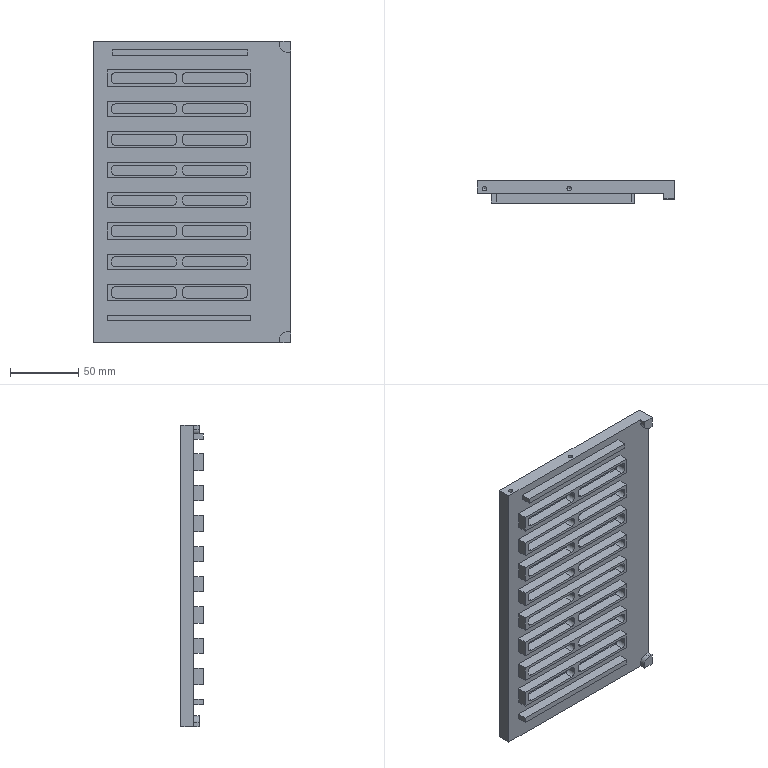NC program | NX | posted with a generic post | part box 144.5 x 16.5 x 221 mm
Lines 25 to 834 of 8751:
(动态加工0.5 , TOOL : D8-25-D8-60-3T-ROUGH)
N48 T02 M6
N50 G53
N52 G17 G0 G90 X-126.572 Y2.423 B0. C0. S6000 M3
N54 G43 Z20. H2
N56 Z-12.
N58 G94 G1 X-126.422 Y2.436 Z-12.937 F3500.
N60 X-126.273 Y2.448 Z-13.308
N62 X-126.123 Y2.46 Z-13.58
N64 X-125.974 Y2.473 Z-13.8
N66 X-125.824 Y2.485 Z-13.984
N68 X-125.675 Y2.497 Z-14.142
N70 X-125.525 Y2.509 Z-14.28
N72 X-125.376 Y2.522 Z-14.4
N74 X-125.226 Y2.534 Z-14.505
N76 X-125.077 Y2.546 Z-14.598
N78 X-124.927 Y2.559 Z-14.679
N80 X-124.778 Y2.571 Z-14.75
N82 X-124.628 Y2.583 Z-14.81
N84 X-124.479 Y2.596 Z-14.862
N86 X-124.329 Y2.608 Z-14.905
N88 X-124.18 Y2.62 Z-14.939
N90 X-124.03 Y2.632 Z-14.966
N92 X-123.881 Y2.645 Z-14.985
N94 X-123.731 Y2.657 Z-14.996
N96 X-123.582 Y2.669 Z-15.
N98 X-122.198 Y2.783
N100 G3 X-121.548 Y3.214 R0.809
N102 X-120.82 Y5.812 R7.175
N104 X-120.527 Y11.884 R57.317
N106 G1 X-120.499 Y20.852
N108 X-120.498 Y76.502
N110 G2 X-119.038 Y79.444 R4.189
N112 X-115.307 Y81.289 R8.348
N114 X-109.801 Y81.906 R27.841
N116 X-97.202 Y81.998 R442.635
N118 G1 X115.027 Y81.997
N120 G2 X118.015 Y80.473 R4.207
N122 X119.814 Y76.725 R8.506
N124 X120.407 Y71.291 R28.543
N126 X120.498 Y58.767 R445.831
N128 G1 Y-76.524
N130 G2 X118.974 Y-79.512 R4.21
N132 X115.292 Y-81.296 R8.462
N134 X109.785 Y-81.907 R28.074
N136 X97.261 Y-81.998 R443.425
N138 G1 X-115.074 Y-81.996
N140 G2 X-118.046 Y-80.436 R4.252
N142 X-119.809 Y-76.741 R8.541
N144 X-120.406 Y-71.308 R28.316
N146 X-120.498 Y-58.783 R440.931
N148 G1 X-120.497 Y0.042
N150 G2 X-120.074 Y3.928 R35.862
N152 G3 X-119.543 Y12.571 R72.923
N154 X-119.499 Y22.428 R692.354
N156 G1 X-119.498 Y73.828
N158 G2 X-117.119 Y78.386 R5.853
N160 X-112.81 Y80.274 R10.684
N162 X-106.701 Y80.904 R34.296
N164 X-94.327 Y80.997 R453.189
N166 G1 X112.476 Y80.994
N168 G2 X116.942 Y78.556 R5.865
N170 X118.82 Y74.1 R10.921
N172 X119.416 Y67.837 R36.785
N174 X119.498 Y55.387 R532.275
N176 G1 X119.494 Y-73.973
N178 G2 X117.007 Y-78.477 R5.893
N180 X112.541 Y-80.332 R11.039
N182 X106.276 Y-80.918 R37.482
N184 X93.827 Y-80.997 R545.572
N186 G1 X-112.473 Y-80.994
N188 G2 X-116.98 Y-78.505 R5.892
N190 X-118.833 Y-74.038 R11.051
N192 X-119.42 Y-67.698 R37.896
N194 X-119.498 Y-55.248 R562.114
N196 G1 X-119.497 Y-2.098
N198 G2 X-119.043 Y3.975 R62.156
N200 G3 X-118.518 Y16.146 R127.55
N202 G1 X-118.499 Y24.377
N204 X-118.497 Y71.577
N206 G2 X-115.243 Y77.527 R6.962
N208 X-110.43 Y79.342 R12.909
N210 X-103.862 Y79.917 R42.826
N212 X-91.113 Y79.997 R580.954
N214 G1 X110.062 Y79.996
N216 G2 X115.98 Y76.819 R6.934
N218 X117.811 Y72.095 R12.632
N220 X118.419 Y65.304 R42.014
N222 X118.497 Y52.555 R594.339
N224 G1 Y-71.52
N226 G2 X115.257 Y-77.521 R6.958
N228 X110.437 Y-79.34 R12.859
N230 X103.869 Y-79.916 R42.675
N232 X91.044 Y-79.997 R572.005
N234 G1 X-109.981
N236 G2 X-116.086 Y-76.658 R6.99
N238 X-117.847 Y-71.902 R13.06
N240 X-118.417 Y-65.333 R42.909
N242 X-118.497 Y-52.959 R565.196
N244 G1 X-118.496 Y-3.823
N246 G2 X-118.029 Y4.001 R89.068
N248 G3 X-117.515 Y17.567 R166.648
N250 G1 X-117.5 Y25.802
N252 X-117.498 Y69.402
N254 G2 X-116.518 Y73.666 R8.362
N256 X-112.306 Y77.273 R8.771
N258 X-106.93 Y78.592 R18.736
N260 X-98.543 Y78.972 R83.321
N262 G1 X-88.643 Y78.997
N264 X107.901 Y78.996
N266 G2 X112.032 Y78.093 R8.448
N268 X115.653 Y74.066 R8.574
N270 X117.076 Y68.568 R18.105
N272 X117.471 Y60.181 R80.674
N274 G1 X117.497 Y50.281
N276 X117.496 Y-69.398
N278 G2 X116.595 Y-73.53 R8.459
N280 X112.602 Y-77.139 R8.605
N282 X107.184 Y-78.561 R17.911
N284 X99.398 Y-78.962 R73.9
N286 G1 X88.673 Y-78.997
N288 X-107.974 Y-78.996
N290 G2 X-112.355 Y-77.908 R8.215
N292 X-115.794 Y-73.751 R8.867
N294 X-117.123 Y-68.148 R19.381
N296 X-117.471 Y-60.133 R86.468
N298 G1 X-117.497 Y-50.233
N300 X-117.496 Y-5.283
N302 G2 X-117.03 Y3.898 R114.608
N304 G3 X-116.507 Y20.185 R214.532
N306 G1 X-116.5 Y26.777
N308 X-116.497 Y67.677
N310 G2 X-115.77 Y71.707 R9.891
N312 X-114.392 Y73.841 R8.626
N314 X-113.812 Y74.84 R9.182
N316 G1 X-113.166 Y75.506
N318 X-112.382 Y76.016
N320 G2 X-104.826 Y77.671 R26.45
N322 X-94.784 Y77.982 R129.687
N324 G1 X-86.234 Y77.996
N326 X105.941 Y77.995
N328 G2 X109.85 Y77.416 R10.756
N330 X112.046 Y76.145 R8.329
N332 X114.414 Y73.807 R4.347
N334 X116.017 Y67.661 R21.369
N336 X116.455 Y59.576 R76.219
N338 X116.497 Y47.952 R776.314
N340 G1 X116.496 Y-67.423
N342 G2 X115.925 Y-71.334 R10.852
N344 X114.389 Y-73.845 R8.349
N346 X113.795 Y-74.854 R8.385
N348 G1 X113.129 Y-75.525
N350 X112.331 Y-76.03
N352 G2 X104.54 Y-77.691 R27.089
N354 X95.097 Y-77.981 R129.679
N356 G1 X85.647 Y-77.996
N358 X-105.928 Y-77.995
N360 G2 X-109.838 Y-77.421 R10.811
N362 X-112.065 Y-76.134 R8.669
N364 X-113.117 Y-75.535 R5.064
N366 G1 X-113.431 Y-75.318
N368 G2 X-114.645 Y-73.254 R6.134
N370 X-116.102 Y-66.911 R23.207
N372 X-116.475 Y-57.847 R98.48
N374 G1 X-116.497 Y-48.772
N376 X-116.495 Y-6.448
N378 G2 X-115.991 Y4.399 R154.223
N380 G3 X-115.507 Y22.284 R267.315
N382 G1 X-115.5 Y29.478
N384 X-115.499 Y65.428
N386 G2 X-115.121 Y69.297 R14.61
N388 G1 X-114.705 Y70.58
N390 G2 X-114.674 Y72.714 R53.083
N392 X-114.306 Y74.023 R5.537
N394 G1 X-114.597 Y73.172
N396 G3 X-114.7 Y72.25 R4.874
N398 G2 X-114.826 Y67.431 R63.555
N400 G3 X-114.9 Y56.482 R427.272
N402 G1 X-114.902 Y26.224
N404 G2 X-115.149 Y8.97 R408.984
N406 X-115.735 Y-1.084 R927.803
N408 G3 X-115.895 Y-10.982 R203.441
N410 G1 X-115.896 Y-69.082
N412 X-115.907 Y-69.211
N414 X-115.938 Y-69.338
N416 X-115.99 Y-69.457
N418 X-116.87 Y-70.751 Z-14.8
N420 X-117.517 Y-71.697 F15000.
N422 G3 X-117.656 Y-72.13 R0.814
N424 G1 X-117.68 Y-73.17
N426 G3 X-117.306 Y-73.866 R0.801
N428 G1 X-116.187 Y-74.568
N430 X-115.775 Y-74.83 Z-14.862 F3500.
N432 X-115.356 Y-75.079 Z-14.925
N434 G3 X-114.781 Y-75.106 Z-15. R0.82
N436 X-114.28 Y-74.081 R0.8
N438 G1 X-114.594 Y-73.189
N440 G2 X-114.709 Y-71.121 R12.101
N442 X-114.891 Y-62.061 R153.374
N444 G1 X-114.896 Y-55.461
N446 Y66.539
N448 G3 X-115.166 Y67.138 R0.803
N450 X-115.993 Y67.285 Z-14.887 R0.828
N452 G1 X-116.648 Y67.094 Z-14.8
N454 X-117.85 Y66.742 F15000.
N456 G2 X-117.945 Y68.299 R-0.8
N458 G3 X-117.48 Y68.268 R1.327
N460 X-116.877 Y68.756 R0.801
N462 G1 X-116.667 Y69.276
N464 X-116.437 Y69.853 Z-14.879 F3500.
N466 X-116.195 Y70.424 Z-14.959
N468 X-116.099 Y70.554 Z-14.979
N470 X-115.983 Y70.665 Z-15.
N472 G2 X-114.7 Y70.027 R0.8
N474 G1 Y-72.25
N476 X-114.594 Y-73.189
N478 G3 X-113.907 Y-74.735 R5.716
N480 G1 X-113.431 Y-75.318
N482 X-112.321 Y-76.035
N484 G3 X-105.433 Y-77.31 R20.765
N486 X-94.184 Y-77.396 R367.013
N488 G1 X107.316
N490 X107.446 Y-77.407
N492 X107.572 Y-77.438
N494 X107.692 Y-77.49
N496 G2 X108.119 Y-78.223 Z-14.886 R0.827
N498 G1 X108.159 Y-78.894 Z-14.8
N500 X108.232 Y-80.132 F15000.
N502 G3 X109.805 Y-79.885 R-0.8
N504 G1 X109.724 Y-79.575
N506 X109.657 Y-79.262
N508 G2 X110.257 Y-78.415 R0.813
N510 G1 X111.739 Y-77.912 Z-15. F3500.
N512 G3 X111.439 Y-76.344 R0.801
N514 G1 X110.499 Y-76.45
N516 X-110.501
N518 X-111.578 Y-76.344
N520 X-114.012 Y-76.94
N522 G2 X-114.793 Y-76.715 R0.809
N524 G1 X-114.897 Y-76.606 Z-14.996
N526 X-115.001 Y-76.498 Z-14.985
N528 X-115.104 Y-76.39 Z-14.966
N530 X-115.208 Y-76.281 Z-14.939
N532 X-115.312 Y-76.173 Z-14.905
N534 X-115.415 Y-76.064 Z-14.862
N536 X-115.519 Y-75.956 Z-14.81
N538 X-115.623 Y-75.847 Z-14.75
N540 X-115.726 Y-75.739 Z-14.679
N542 X-115.83 Y-75.63 Z-14.598
N544 X-115.933 Y-75.522 Z-14.505
N546 X-116.037 Y-75.414 Z-14.4
N548 X-116.141 Y-75.305 Z-14.28
N550 X-116.244 Y-75.197 Z-14.142
N552 X-116.348 Y-75.088 Z-13.984
N554 X-116.452 Y-74.98 Z-13.8
N556 X-116.555 Y-74.871 Z-13.58
N558 X-116.659 Y-74.763 Z-13.308
N560 X-116.763 Y-74.655 Z-12.937
N562 X-116.866 Y-74.546 Z-12.
N564 G0 Z20.
N566 X-110.132 Y78.917
N568 Z-12.
N570 G1 X-110.273 Y78.866 Z-12.937
N572 X-110.414 Y78.814 Z-13.308
N574 X-110.555 Y78.763 Z-13.58
N576 X-110.696 Y78.712 Z-13.8
N578 X-110.837 Y78.66 Z-13.984
N580 X-110.978 Y78.609 Z-14.142
N582 X-111.119 Y78.558 Z-14.28
N584 X-111.26 Y78.506 Z-14.4
N586 X-111.401 Y78.455 Z-14.505
N588 X-111.542 Y78.404 Z-14.598
N590 X-111.683 Y78.352 Z-14.679
N592 X-111.824 Y78.301 Z-14.75
N594 X-111.965 Y78.25 Z-14.81
N596 X-112.106 Y78.198 Z-14.862
N598 X-112.247 Y78.147 Z-14.905
N600 X-112.388 Y78.096 Z-14.939
N602 X-112.528 Y78.044 Z-14.966
N604 X-112.669 Y77.993 Z-14.985
N606 X-112.81 Y77.942 Z-14.996
N608 X-112.951 Y77.89 Z-15.
N610 G3 X-112.67 Y76.323 R0.808
N612 X-110.538 Y76.45 R10.828
N614 X-105.599 Y76.621 R42.041
N616 G2 X-92.557 Y76.984 R193.286
N618 G1 X-83.707 Y76.996
N620 X106.093 Y76.988
N622 G2 X108.504 Y76.455 R13.506
N624 G1 X110.501 Y76.45
N626 G2 X112.067 Y76.135 R4.094
N628 G3 X110.501 Y76.45 R4.094
N630 G1 X-108.2
N632 G2 X-108.545 Y76.527 R0.864
N634 G1 X-109.265 Y76.866
N636 G2 X-108.921 Y78.405 R0.808
N638 G1 X-108.771 Z-14.996
N640 X-108.621 Z-14.985
N642 X-108.471 Z-14.966
N644 X-108.321 Z-14.939
N646 X-108.171 Z-14.905
N648 X-108.021 Z-14.862
N650 X-107.871 Z-14.81
N652 X-107.721 Z-14.75
N654 X-107.571 Z-14.679
N656 X-107.421 Z-14.598
N658 X-107.271 Z-14.505
N660 X-107.121 Z-14.4
N662 X-106.971 Z-14.28
N664 X-106.821 Z-14.142
N666 X-106.671 Z-13.984
N668 X-106.521 Z-13.8
N670 X-106.371 Z-13.58
N672 X-106.221 Z-13.308
N674 X-106.071 Z-12.937
N676 X-105.921 Z-12.
N678 G0 Z20.
N680 X112.849 Y78.683
N682 Z-12.
N684 G1 X112.953 Y78.575 Z-12.937
N686 X113.056 Y78.466 Z-13.308
N688 X113.16 Y78.357 Z-13.58
N690 X113.263 Y78.249 Z-13.8
N692 X113.367 Y78.14 Z-13.984
N694 X113.47 Y78.032 Z-14.142
N696 X113.574 Y77.923 Z-14.28
N698 X113.677 Y77.814 Z-14.4
N700 X113.781 Y77.706 Z-14.505
N702 X113.884 Y77.597 Z-14.598
N704 X113.987 Y77.489 Z-14.679
N706 X114.091 Y77.38 Z-14.75
N708 X114.194 Y77.271 Z-14.81
N710 X114.298 Y77.163 Z-14.862
N712 X114.401 Y77.054 Z-14.905
N714 X114.505 Y76.946 Z-14.939
N716 X114.608 Y76.837 Z-14.966
N718 X114.712 Y76.728 Z-14.985
N720 X114.815 Y76.62 Z-14.996
N722 X114.919 Y76.511 Z-15.
N724 G2 X114.813 Y75.303 R0.808
N726 G1 X114.616 Y75.16
N728 X114.428 Y75.006
N730 G3 X114.255 Y74.146 R0.809
N732 G2 X114.7 Y72.589 R4.894
N734 G3 X114.91 Y68.872 R26.258
N736 G2 X115.47 Y56.739 R125.425
N738 G1 X115.496 Y45.49
N740 X115.489 Y-68.399
N742 G2 X114.718 Y-70.746 R15.407
N744 G3 X114.7 Y-72.756 R32.963
N746 G2 X114.323 Y-73.978 R4.614
N748 G3 X114.7 Y-72.756 R4.614
N750 G2 X114.814 Y-68.647 R44.469
N752 G3 X114.896 Y-57.548 R380.538
N754 G1 X114.888 Y67.402
N756 X114.7 Y68.1
N758 Y71.325
N760 Y-70.575
N762 G3 X115.489 Y-71.383 R0.808
N764 G1 X116.656 Y-71.41
N766 X116.806 Y-71.414 Z-14.996
N768 X116.956 Y-71.418 Z-14.985
N770 X117.106 Y-71.421 Z-14.966
N772 X117.256 Y-71.425 Z-14.939
N774 X117.406 Y-71.428 Z-14.905
N776 X117.556 Y-71.432 Z-14.862
N778 X117.706 Y-71.435 Z-14.81
N780 X117.855 Y-71.439 Z-14.75
N782 X118.005 Y-71.442 Z-14.679
N784 X118.155 Y-71.446 Z-14.598
N786 X118.305 Y-71.449 Z-14.505
N788 X118.455 Y-71.453 Z-14.4
N790 X118.605 Y-71.456 Z-14.28
N792 X118.755 Y-71.46 Z-14.142
N794 X118.905 Y-71.464 Z-13.984
N796 X119.055 Y-71.467 Z-13.8
N798 X119.205 Y-71.471 Z-13.58
N800 X119.355 Y-71.474 Z-13.308
N802 X119.505 Y-71.478 Z-12.937
N804 X119.655 Y-71.481 Z-12.
N806 G0 Z20.
N808 X3.098 Y-2.223
N810 Z3.
N812 G3 X3.098 Y-2.223 Z2.605 I-3.098 J1.833
N814 X3.098 Y-2.223 Z2.21 I-3.098 J1.833
N816 X3.098 Y-2.223 Z1.816 I-3.098 J1.833
N818 X3.098 Y-2.223 Z1.421 I-3.098 J1.833
N820 X3.098 Y-2.223 Z1.026 I-3.098 J1.833
N822 X3.098 Y-2.223 Z0.631 I-3.098 J1.833
N824 X3.098 Y-2.223 Z0.236 I-3.098 J1.833
N826 X3.098 Y-2.223 Z-0.159 I-3.098 J1.833
N828 X3.098 Y-2.223 Z-0.553 I-3.098 J1.833
N830 X3.098 Y-2.223 Z-0.948 I-3.098 J1.833
N832 X3.098 Y-2.223 Z-1.343 I-3.098 J1.833
N834 X3.098 Y-2.223 Z-1.738 I-3.098 J1.833
N836 X3.098 Y-2.223 Z-2.133 I-3.098 J1.833
N838 X3.098 Y-2.223 Z-2.528 I-3.098 J1.833
N840 X3.098 Y-2.223 Z-2.922 I-3.098 J1.833
N842 X3.098 Y-2.223 Z-3.317 I-3.098 J1.833
N844 X3.098 Y-2.223 Z-3.712 I-3.098 J1.833
N846 X3.098 Y-2.223 Z-4.107 I-3.098 J1.833
N848 X3.098 Y-2.223 Z-4.502 I-3.098 J1.833
N850 X3.098 Y-2.223 Z-4.896 I-3.098 J1.833
N852 X3.098 Y-2.223 Z-5.291 I-3.098 J1.833
N854 X3.098 Y-2.223 Z-5.686 I-3.098 J1.833
N856 X3.098 Y-2.223 Z-6.081 I-3.098 J1.833
N858 X3.098 Y-2.223 Z-6.476 I-3.098 J1.833
N860 X3.098 Y-2.223 Z-6.871 I-3.098 J1.833
N862 X3.098 Y-2.223 Z-7.265 I-3.098 J1.833
N864 X3.6 Y-0.39 Z-7.299 R3.6
N866 X-1.006 Y-3.893 R-3.622
N868 X2.928 Y-2.599 R3.686
N870 X0.479 Y3.685 R3.793
N872 X2.236 Y-3.893 R-4.131
N874 X3.065 Y3.008 R4.366
N876 X-4.467 Y-1.725 R4.609
N878 X3.209 Y-3.861 R4.73
N880 X-0.297 Y4.786 R4.92
N882 X0.926 Y-5.552 R-5.215
N884 X-0.408 Y5.36 R5.503
N886 X0.134 Y-6.216 R5.796
N888 X0.058 Y5.974 R6.096
N890 X-0.221 Y-6.824 R6.401
N892 X0.299 Y6.591 R6.712
N894 X-0.611 Y-7.432 R7.028
N896 X1.149 Y7.146 R7.347
N898 X-4.379 Y-6.733 R7.66
N900 X7.94 Y1.018 R7.942
N902 X-4.099 Y6.863 R8.118
N904 X0.521 Y-8.786 R8.375
N906 X2.856 Y8.093 R8.685
N908 X-7.728 Y-5.109 R8.988
N910 X7.836 Y-5.318 R9.222
N912 X-2.382 Y9.02 R9.448
N914 X-2.533 Y-9.845 R9.748
N916 X8.079 Y5.941 R10.056
N918 X-9.146 Y4.67 R10.301
N920 X3.381 Y-10.4 R10.526
N922 X3.121 Y10.259 R10.829
N924 X-9.436 Y-6.434 R11.135
N926 X9.333 Y-6.974 R11.384
N928 X-2.58 Y11.216 R11.625
N930 X-6.196 Y-10.631 R11.929
N932 X12.155 Y1.854 R12.207
N934 X-8.87 Y8.647 R12.446
N936 X-4.574 Y-12.283 R12.712
N938 X11.582 Y5.937 R13.001
N940 X-10.837 Y7.557 R13.256
N942 X1.677 Y-13.84 R13.513
N944 X8.901 Y10.481 R13.816
N946 X-13.681 Y3.506 R14.086
N948 X7.269 Y-12.817 R14.345
N950 X3.495 Y14.099 R14.643
N952 X-14.135 Y-5.446 R14.921
N954 X11.823 Y-10.024 R15.17
N956 X2.175 Y15.168 R15.459
N958 X-14.473 Y-6.75 R15.728
N960 X12.884 Y-9.977 R15.978
N962 X1.099 Y16.088 R16.266
N964 X-15.248 Y-6.974 R16.538
N966 X14.02 Y-9.776 R16.777
N968 X0.723 Y16.916 R17.073
N970 X-16.143 Y-6.923 R17.347
N972 X15.245 Y-9.372 R17.593
N974 X0.133 Y17.746 R17.894
N976 X-17.555 Y-5.273 R18.152
N978 X16.098 Y-9.532 R18.396
N980 X0.708 Y18.543 R18.706
N982 X-18.314 Y-5.586 R18.957
N984 X16.852 Y-9.869 R19.209
N986 X0.54 Y19.371 R19.528
N988 X-19.258 Y-5.247 R19.787
N990 X17.997 Y-9.503 R20.039
N992 X-1.453 Y20.169 R20.369
N994 X-20.231 Y-4.724 R20.622
N996 X19.274 Y-8.766 R20.87
N998 X-0.855 Y21.031 R21.202
N1000 X-21.486 Y-1.518 R21.424
N1002 X18.921 Y-11.293 R21.692
N1004 X-1.162 Y21.855 R22.044
N1006 X-22.337 Y-1.167 R22.255
N1008 X17.608 Y-14.654 R22.522
N1010 X-1.937 Y22.65 R22.888
N1012 X-23.179 Y-1.269 R23.107
N1014 X18.328 Y-15.12 R23.37
N1016 X-1.634 Y23.518 R23.738
N1018 X-23.975 Y1.335 R23.928
N1020 X16.446 Y-18.341 R24.207
N1022 X-0.774 Y24.404 R24.578
N1024 X-24.583 Y3.463 R24.755
N1026 X13.669 Y-21.536 R25.048
N1028 X7.185 Y24.186 R25.399
N1030 X-25.032 Y5.59 R25.567
N1032 X10.46 Y-24.211 R25.895
N1034 X22.347 Y13.518 R26.208
N1036 X-25.806 Y6.041 R26.413
N1038 X11.242 Y-24.812 R26.757
N1040 X23.218 Y13.739 R27.071
N1042 X-26.301 Y7.494 R27.272
N1044 X11.629 Y-25.59 R27.622
N1046 X23.412 Y15.059 R27.935
N1048 X-26.966 Y8.274 R28.139
N1050 X11.632 Y-26.544 R28.49
N1052 X24.124 Y15.555 R28.799
N1054 X-27.059 Y10.554 R28.997
N1056 X7.878 Y-28.794 R29.349
N1058 X25.049 Y15.724 R29.647
N1060 X-28.257 Y9.877 R29.879
N1062 X8.207 Y-29.614 R30.225
N1064 X24.479 Y18.092 R30.525
N1066 X-29.323 Y9.493 R30.763
N1068 X12.823 Y-28.898 R31.115
N1070 X21.853 Y22.405 R31.428
N1072 X-29.654 Y11.141 R31.633
N1074 X10.279 Y-30.826 R31.985
N1076 X22.194 Y23.293 R32.296
N1078 X-30.293 Y11.925 R32.518
N1080 X16.089 Y-29.246 R32.883
N1082 X17.743 Y27.873 R33.208
N1084 X-30.552 Y13.547 R33.394
N1086 X14.853 Y-30.881 R33.762
N1088 X18.424 Y28.488 R34.088
N1090 X-30.926 Y14.826 R34.289
N1092 X13.312 Y-32.539 R34.645
N1094 X20.368 Y28.237 R34.966
N1096 X-31.462 Y15.732 R35.179
N1098 X12.096 Y-33.958 R35.53
N1100 X21.944 Y28.176 R35.852
N1102 X-32.205 Y16.24 R36.092
N1104 X12.526 Y-34.753 R36.423
N1106 X22.616 Y28.784 R36.745
N1108 X-32.551 Y17.488 R36.988
N1110 X14.684 Y-34.871 R37.32
N1112 X21.242 Y30.898 R37.648
N1114 X-36.541 Y10.207 R37.896
N1116 X16.114 Y-35.222 R38.222
N1118 X21. Y32.138 R38.549
N1120 X-37.602 Y9.752 R38.797
N1122 X16.843 Y-35.875 R39.122
N1124 X20.813 Y33.323 R39.451
N1126 X-39.091 Y7.341 R39.7
N1128 X15.605 Y-37.409 R40.016
N1130 X23.007 Y32.956 R40.344
N1132 X-39.642 Y9.021 R40.595
N1134 X14.251 Y-38.906 R40.908
N1136 X25.215 Y32.454 R41.238
N1138 X-40.307 Y10.072 R41.493
N1140 X9.386 Y-41.279 R41.8
N1142 X28.473 Y30.886 R42.127
N1144 X-40.537 Y12.512 R42.389
N1146 X5.686 Y-42.853 R42.694
N1148 X33.469 Y26.886 R43.01
N1150 X-40.643 Y14.944 R43.283
N1152 X2.609 Y-44.047 R43.59
N1154 X35.827 Y25.279 R43.905
N1156 X-40.929 Y16.67 R44.186
N1158 X0.967 Y-45.017 R44.492
N1160 X37.253 Y24.812 R44.808
N1162 X-40.551 Y19.674 R45.088
N1164 X-0.635 Y-45.926 R45.396
N1166 X39.016 Y23.751 R45.711
N1168 X-40.027 Y22.567 R45.987
N1170 X-5.883 Y-46.449 R46.291
N1172 X42.387 Y19.383 R46.603
N1174 X-40.201 Y24.055 R46.89
N1176 X-7.34 Y-47.157 R47.198
N1178 X43.853 Y18.321 R47.509
N1180 X-40.825 Y24.785 R47.803
N1182 X-2.626 Y-48.586 R48.117
N1184 X42.291 Y23.572 R48.438
N1186 X-42.322 Y24.061 R48.721
N1188 X-5.284 Y-49.279 R49.024
N1190 X44.738 Y20.812 R49.342
N1192 X-41.933 Y26.453 R49.632
N1194 X-5.47 Y-50.18 R49.94
N1196 X45.688 Y20.944 R50.257
N1198 X-42.859 Y26.701 R50.547
N1200 X-6.209 Y-51.015 R50.853
N1202 X46.864 Y20.569 R51.172
N1204 X-43.068 Y28.062 R51.461
N1206 X-7.492 Y-51.765 R51.767
N1208 X47.933 Y20.415 R52.087
N1210 X-42.486 Y30.503 R52.377
N1212 X-6.942 Y-52.77 R52.686
N1214 X48.572 Y21.246 R53.007
N1216 X-42.472 Y32.053 R53.293
N1218 X-8.466 Y-53.472 R53.601
N1220 X50.036 Y20.149 R53.921
N1222 X-43.61 Y32.075 R54.213
N1224 X-8.087 Y-54.463 R54.522
N1226 X50.104 Y22.326 R54.844
N1228 X-43.48 Y33.757 R55.134
N1230 X-12.967 Y-54.439 R55.438
N1232 X53.31 Y16.481 R55.75
N1234 X-42.48 Y36.406 R56.046
N1236 X-13.516 Y-55.255 R56.357
N1238 X53.286 Y19.415 R56.678
N1240 X-43.827 Y36.249 R56.974
N1242 X-15.288 Y-55.74 R57.277
N1244 X55.247 Y16.467 R57.593
N1246 X-42.143 Y39.52 R57.889
N1248 X-17.469 Y-56.054 R58.196
N1250 X56.723 Y14.639 R58.511
N1252 X-41.187 Y41.8 R58.807
N1254 X-20.034 Y-56.161 R59.114
N1256 X58.215 Y12.377 R59.43
N1258 X-41.722 Y42.569 R59.729
N1260 X-19.778 Y-57.235 R60.041
N1262 X58.826 Y13.86 R60.358
N1264 X-41.991 Y43.594 R60.656
N1266 X-21.464 Y-57.606 R60.964
N1268 X60.081 Y12.504 R61.28
N1270 X-41.995 Y44.86 R61.577
N1272 X-22.677 Y-58.13 R61.888
N1274 X61.203 Y11.635 R62.205
N1276 X51.177 Y35.38 R62.396
N1278 X4.468 Y62.05 R62.355
N1280 G1 X-4.508 Y62.035
N1282 G3 X-46.275 Y41.911 R62.426
N1284 X-29.317 Y-56.098 R62.821
N1286 G1 X-28.789 Y-56.17
N1288 X-27.626 Y-56.523
N1290 G2 X-25.412 Y-57.786 R41.415
N1292 G3 X-17.518 Y-60.894 R41.797
N1294 X-6.758 Y-63.05 R62.457
N1296 G1 X6.142
N1298 G3 X20.066 Y-60.206 R56.099
N1300 X25.293 Y-58.193 R59.821
N1302 X25.617 Y-57.865 R2.237
N1304 G1 X26.557 Y-57.094
N1306 X27.629 Y-56.522
N1308 G3 X32.541 Y-54.405 R20.393
N1310 X47.527 Y-42.014 R59.821
N1312 X11.698 Y62.05 R63.357
N1314 G1 X4.423
N1316 G2 X13.318 Y62.034 R603.781
N1318 X18.439 Y60.96 R26.285
N1320 X26.03 Y58.136 R59.403
N1322 G1 X26.262 Y57.963
N1324 G3 X29.35 Y56.507 R270.074
N1326 G2 X57.984 Y26.527 R63.474
N1328 X35.947 Y-52.956 R63.741
N1330 X30.527 Y-56.021 R34.543
N1332 X30.001 Y-56.05 R3.253
N1334 G1 X28.792 Y-56.169
N1336 G2 X31.107 Y-56.038 R16.684
N1338 G3 X34.223 Y-54.949 R9.769
N1340 X41.157 Y-50.254 R40.939
N1342 X50.57 Y40.336 R64.8
N1344 X30.458 Y56.99 R63.463
N1346 X29.499 Y57.05 R2.997
N1348 G1 X28.37 Y57.154
N1350 X27.279 Y57.462
N1352 X28.37 Y57.154
N1354 G3 X30.424 Y57.048 R12.965
N1356 G2 X32.887 Y56.163 R8.204
N1358 X40.042 Y51.493 R46.092
N1360 X43.242 Y-49.232 R65.394
N1362 X35.513 Y-54.86 R47.068
N1364 X32.892 Y-56.042 R13.804
N1366 G1 X30.944 Y-56.05
N1368 G3 X33.83 Y-56.027 R42.761
N1370 X37.056 Y-54.841 R10.027
N1372 X43.585 Y-50.179 R38.581
N1374 X60.674 Y26.573 R66.197
N1376 X36.981 Y54.847 R65.835
N1378 X33.122 Y57.012 R27.059
N1380 G1 X32.923 Y57.05
N1382 X30.298
N1384 G2 X33.331 Y57.03 R56.648
N1386 X36.109 Y55.935 R9.264
N1388 X43.14 Y50.937 R45.641
N1390 X45.825 Y-48.933 R66.904
N1392 X38.407 Y-54.681 R45.623
N1394 X35.475 Y-56.061 R14.353
N1396 X33.501 Y-56.05 R97.387
N1398 X35.976 Y-56.118 R21.79
N1400 G3 X38.886 Y-55.216 R7.577
N1402 X44.493 Y-51.357 R30.133
N1404 X59.983 Y-31.935 R65.68
N1406 X41.803 Y53.238 R67.856
N1408 X36.289 Y56.826 R33.601
N1410 X35.409 Y57.133 R2.182
N1412 G2 X33.074 Y57.05 R16.229
N1414 G3 X35.633 Y57.15 R15.646
N1416 G2 X37.878 Y56.42 R6.296
N1418 X43.099 Y52.92 R31.266
N1420 X66.236 Y16.911 R68.102
N1422 X47.168 Y-49.738 R68.226
N1424 X40.638 Y-54.839 R40.512
N1426 X37.124 Y-56.349 R11.735
N1428 G1 X36.848 Y-56.344
N1430 G3 X35.796 Y-56.116 R5.694
N1432 G2 X37.223 Y-56.442 R8.196
N1434 G3 X39.607 Y-56.079 R4.985
N1436 X44.094 Y-53.511 R18.731
N1438 X52.778 Y-45.231 R54.142
N1440 X44.76 Y52.79 R69.35
N1442 X39.167 Y56.722 R34.889
N1444 X37.177 Y57.537 R8.808
N1446 X36.719 Y57.461 R1.126
N1448 G1 X35.553 Y57.147
N1450 G3 X36.892 Y57.546 R6.522
N1452 G2 X38.245 Y57.444 R2.629
N1454 X41.952 Y55.577 R13.817
N1456 X50.31 Y48.398 R53.466
N1458 X51.06 Y-47.992 R69.941
N1460 X43.646 Y-54.488 R46.707
N1462 X39.463 Y-56.594 R15.095
N1464 X37.954 Y-56.79 R3.825
N1466 G1 X37.011 Y-56.385
N1468 G3 X38.379 Y-56.965 R11.036
N1470 X40.946 Y-56.699 R5.057
N1472 X45.319 Y-54.344 R16.935
N1474 X53.077 Y-47.195 R48.503
N1476 X47.602 Y52.327 R70.865
N1478 X41.652 Y56.819 R38.113
N1480 X38.441 Y58.119 R9.919
N1482 X37.736 Y57.961 R0.906
N1484 G1 X36.861 Y57.531
N1486 G3 X37.913 Y58.093 R5.827
N1488 G2 X39.093 Y58.194 R2.046
N1490 X42.307 Y56.958 R9.606
N1492 X47.986 Y52.73 R35.058
N1494 X67.824 Y22.297 R70.775
N1496 X52.473 Y-48.696 R71.273
N1498 X45.298 Y-55.009 R44.292
N1500 X40.933 Y-57.166 R15.098
N1502 X38.837 Y-57.342 R4.876
N1504 X38.02 Y-56.835 R4.239
N1506 G3 X39.067 Y-57.518 R9.88
N1508 X41.368 Y-57.61 R4.188
N1510 X45.455 Y-55.876 R12.811
N1512 X51.826 Y-50.705 R36.364
N1514 X67.455 Y-26.586 R70.277
N1516 X49.839 Y52.328 R72.384
N1518 X43.614 Y57.211 R39.162
N1520 X40.001 Y58.743 R11.536
N1522 X38.947 Y58.796 R2.715
N1524 X38.644 Y58.639 R4.029
N1526 G1 X37.802 Y58.011
N1528 G3 X38.757 Y58.749 R12.255
N1530 G2 X40.005 Y58.965 R2.119
N1532 X43.35 Y57.878 R8.803
N1534 X48.825 Y53.983 R29.741
N1536 X62.631 Y37.278 R69.327
N1538 X55.607 Y-47.47 R72.909
N1540 X47.827 Y-54.912 R49.369
N1542 X42.935 Y-57.645 R18.682
N1544 X39.779 Y-58.025 R6.433
N1546 X39.303 Y-57.82 R1.108
N1548 G1 X38.926 Y-57.452
N1550 G3 X39.75 Y-58.178 R4.015
N1552 X42.066 Y-58.453 R4.075
N1554 X46.341 Y-56.88 R11.907
N1556 X52.565 Y-52.064 R32.585
N1558 X64.496 Y-36.403 R68.064
N1560 X52.169 Y52.191 R73.917
N1562 X45.62 Y57.574 R41.844
N1564 X41.477 Y59.455 R13.634
N1566 X39.621 Y59.535 R4.423
N1568 X39.299 Y59.346 R2.882
N1570 G1 X38.644 Y58.639
N1572 X39.401 Y59.456
N1574 G2 X40.92 Y59.802 R2.447
N1576 X44.447 Y58.772 R8.961
N1578 X49.886 Y55.032 R27.378
N1580 X61.092 Y42.477 R66.911
N1582 X58.159 Y-46.785 R74.486
N1584 X49.977 Y-55.052 R52.869
N1586 X44.723 Y-58.21 R21.494
N1588 X41.234 Y-58.873 R8.353
N1590 X40.002 Y-58.558 R2.558
N1592 X39.71 Y-58.218 R2.321
N1594 G1 X39.496 Y-58.009
N1596 G2 X40.071 Y-58.711 R4.09
N1598 G3 X41.976 Y-59.344 R3.162
N1600 X46.019 Y-58.461 R9.276
N1602 X51.792 Y-54.728 R24.426
N1604 X60.517 Y-45.31 R57.077
N1606 X54.317 Y52.185 R75.418
N1608 X47.493 Y58.014 R44.191
N1610 X42.932 Y60.218 R15.801
N1612 X40.195 Y60.328 R5.402
N1614 X39.761 Y60.018 R1.045
N1616 G1 X39.364 Y59.415
N1618 X39.841 Y60.145
N1620 G2 X40.994 Y60.656 R1.93
N1622 X44.268 Y60.207 R6.894
N1624 X49.44 Y57.264 R20.012
N1626 X57.63 Y49.419 R54.637
N1628 X60.147 Y-46.731 R76.007
N1630 X51.859 Y-55.382 R54.717
N1632 X46.222 Y-58.907 R23.463
N1634 X42.135 Y-59.736 R9.425
N1636 X40.519 Y-59.297 R3.35
N1638 G1 X40.361 Y-59.138
N1640 G2 X40.375 Y-58.357 R0.801
N1642 G1 X41.311 Y-57.104 Z-7.099
N1644 X41.498 Y-56.849 F15000.
N1646 X41.699 Y-56.605
N1648 G2 X42.85 Y-56.649 R0.8
N1650 G1 X43.006 Y-56.821
N1652 X43.151 Y-57.002
N1654 G2 X42.027 Y-58.092 R0.8
N1656 G1 X41.044 Y-57.485 Z-7.247 F3500.
N1658 G3 X40.652 Y-57.391 Z-7.299 R0.812
N1660 X40.021 Y-58.655 R0.8